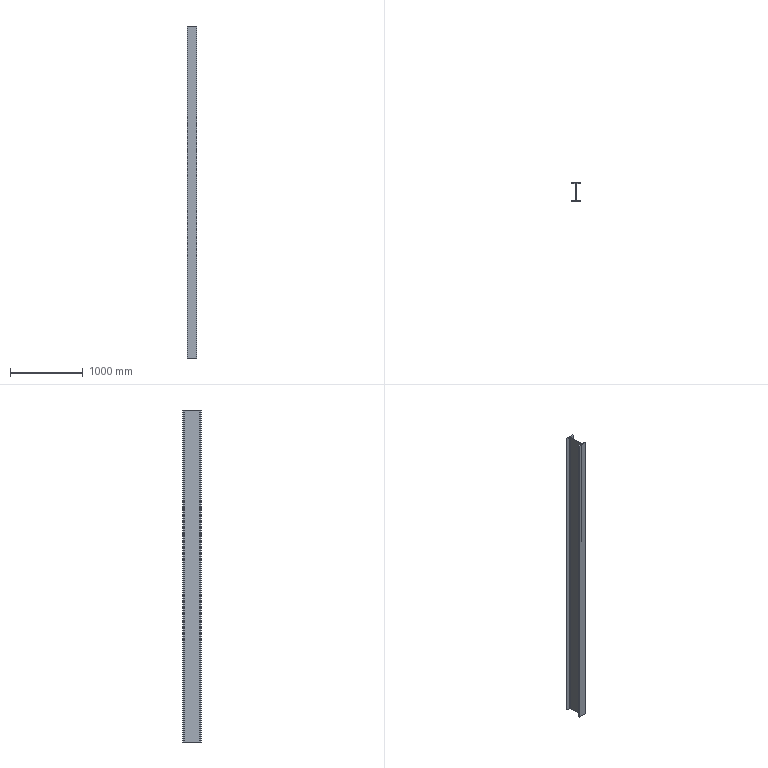Part | SolidWorks | features Extrusion 1 | 1 solid | 18 faces | box 125 x 250 x 4570 mm | volume 16895007 mm3 | plane 14 | cylinder 4 | commonest cylinder face diameters 16 x4
STEP:
#1=CARTESIAN_POINT('',(-62.5,9.,0.));
#2=VERTEX_POINT('',#1);
#3=CARTESIAN_POINT('',(-62.5,0.,0.));
#4=VERTEX_POINT('',#3);
#5=CARTESIAN_POINT('',(-62.5,0.,0.));
#6=DIRECTION('',(0.,-1.,0.));
#7=VECTOR('',#6,1000.);
#8=LINE('',#5,#7);
#9=EDGE_CURVE('',#2,#4,#8,.T.);
#10=ORIENTED_EDGE('',*,*,#9,.T.);
#11=CARTESIAN_POINT('',(-62.5,0.,4570.));
#12=VERTEX_POINT('',#11);
#13=CARTESIAN_POINT('',(-62.5,0.,4570.));
#14=DIRECTION('',(0.,0.,-1.));
#15=VECTOR('',#14,1000.);
#16=LINE('',#13,#15);
#17=EDGE_CURVE('',#12,#4,#16,.T.);
#18=ORIENTED_EDGE('',*,*,#17,.F.);
#19=CARTESIAN_POINT('',(-62.5,9.,4570.));
#20=VERTEX_POINT('',#19);
#21=CARTESIAN_POINT('',(-62.5,0.,4570.));
#22=DIRECTION('',(0.,-1.,0.));
#23=VECTOR('',#22,1000.);
#24=LINE('',#21,#23);
#25=EDGE_CURVE('',#20,#12,#24,.T.);
#26=ORIENTED_EDGE('',*,*,#25,.F.);
#27=CARTESIAN_POINT('',(-62.5,9.,4570.));
#28=DIRECTION('',(0.,0.,-1.));
#29=VECTOR('',#28,1000.);
#30=LINE('',#27,#29);
#31=EDGE_CURVE('',#20,#2,#30,.T.);
#32=ORIENTED_EDGE('',*,*,#31,.T.);
#33=EDGE_LOOP('',(#10,#18,#26,#32));
#34=FACE_OUTER_BOUND('',#33,.T.);
#35=CARTESIAN_POINT('',(-62.5,0.,4570.));
#36=DIRECTION('',(1.,0.,0.));
#37=DIRECTION('',(0.,0.,-1.));
#38=AXIS2_PLACEMENT_3D('',#35,#36,#37);
#39=PLANE('',#38);
#40=ADVANCED_FACE('',(#34),#39,.F.);
#41=CARTESIAN_POINT('',(62.5,0.,0.));
#42=VERTEX_POINT('',#41);
#43=CARTESIAN_POINT('',(62.5,0.,0.));
#44=DIRECTION('',(1.,0.,0.));
#45=VECTOR('',#44,1000.);
#46=LINE('',#43,#45);
#47=EDGE_CURVE('',#4,#42,#46,.T.);
#48=ORIENTED_EDGE('',*,*,#47,.T.);
#49=CARTESIAN_POINT('',(62.5,0.,4570.));
#50=VERTEX_POINT('',#49);
#51=CARTESIAN_POINT('',(62.5,0.,4570.));
#52=DIRECTION('',(0.,0.,-1.));
#53=VECTOR('',#52,1000.);
#54=LINE('',#51,#53);
#55=EDGE_CURVE('',#50,#42,#54,.T.);
#56=ORIENTED_EDGE('',*,*,#55,.F.);
#57=CARTESIAN_POINT('',(62.5,0.,4570.));
#58=DIRECTION('',(1.,0.,0.));
#59=VECTOR('',#58,1000.);
#60=LINE('',#57,#59);
#61=EDGE_CURVE('',#12,#50,#60,.T.);
#62=ORIENTED_EDGE('',*,*,#61,.F.);
#63=ORIENTED_EDGE('',*,*,#17,.T.);
#64=EDGE_LOOP('',(#48,#56,#62,#63));
#65=FACE_OUTER_BOUND('',#64,.T.);
#66=CARTESIAN_POINT('',(62.5,0.,4570.));
#67=DIRECTION('',(0.,1.,0.));
#68=DIRECTION('',(0.,0.,1.));
#69=AXIS2_PLACEMENT_3D('',#66,#67,#68);
#70=PLANE('',#69);
#71=ADVANCED_FACE('',(#65),#70,.F.);
#72=CARTESIAN_POINT('',(62.5,9.,0.));
#73=VERTEX_POINT('',#72);
#74=CARTESIAN_POINT('',(62.5,0.,0.));
#75=DIRECTION('',(0.,1.,0.));
#76=VECTOR('',#75,1000.);
#77=LINE('',#74,#76);
#78=EDGE_CURVE('',#42,#73,#77,.T.);
#79=ORIENTED_EDGE('',*,*,#78,.T.);
#80=CARTESIAN_POINT('',(62.5,9.,4570.));
#81=VERTEX_POINT('',#80);
#82=CARTESIAN_POINT('',(62.5,9.,4570.));
#83=DIRECTION('',(0.,0.,-1.));
#84=VECTOR('',#83,1000.);
#85=LINE('',#82,#84);
#86=EDGE_CURVE('',#81,#73,#85,.T.);
#87=ORIENTED_EDGE('',*,*,#86,.F.);
#88=CARTESIAN_POINT('',(62.5,0.,4570.));
#89=DIRECTION('',(0.,1.,0.));
#90=VECTOR('',#89,1000.);
#91=LINE('',#88,#90);
#92=EDGE_CURVE('',#50,#81,#91,.T.);
#93=ORIENTED_EDGE('',*,*,#92,.F.);
#94=ORIENTED_EDGE('',*,*,#55,.T.);
#95=EDGE_LOOP('',(#79,#87,#93,#94));
#96=FACE_OUTER_BOUND('',#95,.T.);
#97=CARTESIAN_POINT('',(62.5,0.,4570.));
#98=DIRECTION('',(-1.,0.,0.));
#99=DIRECTION('',(0.,0.,1.));
#100=AXIS2_PLACEMENT_3D('',#97,#98,#99);
#101=PLANE('',#100);
#102=ADVANCED_FACE('',(#96),#101,.F.);
#103=CARTESIAN_POINT('',(11.,9.,0.));
#104=VERTEX_POINT('',#103);
#105=CARTESIAN_POINT('',(62.5,9.,0.));
#106=DIRECTION('',(-1.,0.,0.));
#107=VECTOR('',#106,1000.);
#108=LINE('',#105,#107);
#109=EDGE_CURVE('',#73,#104,#108,.T.);
#110=ORIENTED_EDGE('',*,*,#109,.T.);
#111=CARTESIAN_POINT('',(11.,9.,4570.));
#112=VERTEX_POINT('',#111);
#113=CARTESIAN_POINT('',(11.,9.,4570.));
#114=DIRECTION('',(0.,0.,-1.));
#115=VECTOR('',#114,1000.);
#116=LINE('',#113,#115);
#117=EDGE_CURVE('',#112,#104,#116,.T.);
#118=ORIENTED_EDGE('',*,*,#117,.F.);
#119=CARTESIAN_POINT('',(62.5,9.,4570.));
#120=DIRECTION('',(-1.,0.,0.));
#121=VECTOR('',#120,1000.);
#122=LINE('',#119,#121);
#123=EDGE_CURVE('',#81,#112,#122,.T.);
#124=ORIENTED_EDGE('',*,*,#123,.F.);
#125=ORIENTED_EDGE('',*,*,#86,.T.);
#126=EDGE_LOOP('',(#110,#118,#124,#125));
#127=FACE_OUTER_BOUND('',#126,.T.);
#128=CARTESIAN_POINT('',(62.5,9.,4570.));
#129=DIRECTION('',(0.,-1.,0.));
#130=DIRECTION('',(0.,0.,-1.));
#131=AXIS2_PLACEMENT_3D('',#128,#129,#130);
#132=PLANE('',#131);
#133=ADVANCED_FACE('',(#127),#132,.F.);
#134=CARTESIAN_POINT('',(3.,17.,0.));
#135=VERTEX_POINT('',#134);
#136=CARTESIAN_POINT('',(11.,17.,0.));
#137=DIRECTION('',(0.,0.,-1.));
#138=DIRECTION('',(-1.,0.,0.));
#139=AXIS2_PLACEMENT_3D('',#136,#137,#138);
#140=CIRCLE('',#139,8.);
#141=EDGE_CURVE('',#104,#135,#140,.T.);
#142=ORIENTED_EDGE('',*,*,#141,.T.);
#143=CARTESIAN_POINT('',(3.,17.,4570.));
#144=VERTEX_POINT('',#143);
#145=CARTESIAN_POINT('',(3.,17.,4570.));
#146=DIRECTION('',(0.,0.,-1.));
#147=VECTOR('',#146,1000.);
#148=LINE('',#145,#147);
#149=EDGE_CURVE('',#144,#135,#148,.T.);
#150=ORIENTED_EDGE('',*,*,#149,.F.);
#151=CARTESIAN_POINT('',(11.,17.,4570.));
#152=DIRECTION('',(0.,0.,-1.));
#153=DIRECTION('',(-1.,0.,0.));
#154=AXIS2_PLACEMENT_3D('',#151,#152,#153);
#155=CIRCLE('',#154,8.);
#156=EDGE_CURVE('',#112,#144,#155,.T.);
#157=ORIENTED_EDGE('',*,*,#156,.F.);
#158=ORIENTED_EDGE('',*,*,#117,.T.);
#159=EDGE_LOOP('',(#142,#150,#157,#158));
#160=FACE_OUTER_BOUND('',#159,.T.);
#161=CARTESIAN_POINT('',(11.,17.,4570.));
#162=DIRECTION('',(0.,0.,-1.));
#163=DIRECTION('',(-1.,0.,0.));
#164=AXIS2_PLACEMENT_3D('',#161,#162,#163);
#165=CYLINDRICAL_SURFACE('',#164,8.);
#166=ADVANCED_FACE('',(#160),#165,.F.);
#167=CARTESIAN_POINT('',(3.,233.,0.));
#168=VERTEX_POINT('',#167);
#169=CARTESIAN_POINT('',(3.,17.,0.));
#170=DIRECTION('',(0.,1.,0.));
#171=VECTOR('',#170,1000.);
#172=LINE('',#169,#171);
#173=EDGE_CURVE('',#135,#168,#172,.T.);
#174=ORIENTED_EDGE('',*,*,#173,.T.);
#175=CARTESIAN_POINT('',(3.,233.,4570.));
#176=VERTEX_POINT('',#175);
#177=CARTESIAN_POINT('',(3.,233.,4570.));
#178=DIRECTION('',(0.,0.,-1.));
#179=VECTOR('',#178,1000.);
#180=LINE('',#177,#179);
#181=EDGE_CURVE('',#176,#168,#180,.T.);
#182=ORIENTED_EDGE('',*,*,#181,.F.);
#183=CARTESIAN_POINT('',(3.,17.,4570.));
#184=DIRECTION('',(0.,1.,0.));
#185=VECTOR('',#184,1000.);
#186=LINE('',#183,#185);
#187=EDGE_CURVE('',#144,#176,#186,.T.);
#188=ORIENTED_EDGE('',*,*,#187,.F.);
#189=ORIENTED_EDGE('',*,*,#149,.T.);
#190=EDGE_LOOP('',(#174,#182,#188,#189));
#191=FACE_OUTER_BOUND('',#190,.T.);
#192=CARTESIAN_POINT('',(3.,17.,4570.));
#193=DIRECTION('',(-1.,0.,0.));
#194=DIRECTION('',(0.,-1.,0.));
#195=AXIS2_PLACEMENT_3D('',#192,#193,#194);
#196=PLANE('',#195);
#197=ADVANCED_FACE('',(#191),#196,.F.);
#198=CARTESIAN_POINT('',(11.,241.,0.));
#199=VERTEX_POINT('',#198);
#200=CARTESIAN_POINT('',(11.,233.,0.));
#201=DIRECTION('',(0.,0.,-1.));
#202=DIRECTION('',(-1.,0.,0.));
#203=AXIS2_PLACEMENT_3D('',#200,#201,#202);
#204=CIRCLE('',#203,8.);
#205=EDGE_CURVE('',#168,#199,#204,.T.);
#206=ORIENTED_EDGE('',*,*,#205,.T.);
#207=CARTESIAN_POINT('',(11.,241.,4570.));
#208=VERTEX_POINT('',#207);
#209=CARTESIAN_POINT('',(11.,241.,4570.));
#210=DIRECTION('',(0.,0.,-1.));
#211=VECTOR('',#210,1000.);
#212=LINE('',#209,#211);
#213=EDGE_CURVE('',#208,#199,#212,.T.);
#214=ORIENTED_EDGE('',*,*,#213,.F.);
#215=CARTESIAN_POINT('',(11.,233.,4570.));
#216=DIRECTION('',(0.,0.,-1.));
#217=DIRECTION('',(-1.,0.,0.));
#218=AXIS2_PLACEMENT_3D('',#215,#216,#217);
#219=CIRCLE('',#218,8.);
#220=EDGE_CURVE('',#176,#208,#219,.T.);
#221=ORIENTED_EDGE('',*,*,#220,.F.);
#222=ORIENTED_EDGE('',*,*,#181,.T.);
#223=EDGE_LOOP('',(#206,#214,#221,#222));
#224=FACE_OUTER_BOUND('',#223,.T.);
#225=CARTESIAN_POINT('',(11.,233.,4570.));
#226=DIRECTION('',(0.,0.,-1.));
#227=DIRECTION('',(-1.,0.,0.));
#228=AXIS2_PLACEMENT_3D('',#225,#226,#227);
#229=CYLINDRICAL_SURFACE('',#228,8.);
#230=ADVANCED_FACE('',(#224),#229,.F.);
#231=CARTESIAN_POINT('',(62.5,241.,0.));
#232=VERTEX_POINT('',#231);
#233=CARTESIAN_POINT('',(11.,241.,0.));
#234=DIRECTION('',(1.,0.,0.));
#235=VECTOR('',#234,1000.);
#236=LINE('',#233,#235);
#237=EDGE_CURVE('',#199,#232,#236,.T.);
#238=ORIENTED_EDGE('',*,*,#237,.T.);
#239=CARTESIAN_POINT('',(62.5,241.,4570.));
#240=VERTEX_POINT('',#239);
#241=CARTESIAN_POINT('',(62.5,241.,4570.));
#242=DIRECTION('',(0.,0.,-1.));
#243=VECTOR('',#242,1000.);
#244=LINE('',#241,#243);
#245=EDGE_CURVE('',#240,#232,#244,.T.);
#246=ORIENTED_EDGE('',*,*,#245,.F.);
#247=CARTESIAN_POINT('',(11.,241.,4570.));
#248=DIRECTION('',(1.,0.,0.));
#249=VECTOR('',#248,1000.);
#250=LINE('',#247,#249);
#251=EDGE_CURVE('',#208,#240,#250,.T.);
#252=ORIENTED_EDGE('',*,*,#251,.F.);
#253=ORIENTED_EDGE('',*,*,#213,.T.);
#254=EDGE_LOOP('',(#238,#246,#252,#253));
#255=FACE_OUTER_BOUND('',#254,.T.);
#256=CARTESIAN_POINT('',(11.,241.,4570.));
#257=DIRECTION('',(0.,1.,0.));
#258=DIRECTION('',(0.,0.,1.));
#259=AXIS2_PLACEMENT_3D('',#256,#257,#258);
#260=PLANE('',#259);
#261=ADVANCED_FACE('',(#255),#260,.F.);
#262=CARTESIAN_POINT('',(62.5,250.,0.));
#263=VERTEX_POINT('',#262);
#264=CARTESIAN_POINT('',(62.5,241.,0.));
#265=DIRECTION('',(0.,1.,0.));
#266=VECTOR('',#265,1000.);
#267=LINE('',#264,#266);
#268=EDGE_CURVE('',#232,#263,#267,.T.);
#269=ORIENTED_EDGE('',*,*,#268,.T.);
#270=CARTESIAN_POINT('',(62.5,250.,4570.));
#271=VERTEX_POINT('',#270);
#272=CARTESIAN_POINT('',(62.5,250.,4570.));
#273=DIRECTION('',(0.,0.,-1.));
#274=VECTOR('',#273,1000.);
#275=LINE('',#272,#274);
#276=EDGE_CURVE('',#271,#263,#275,.T.);
#277=ORIENTED_EDGE('',*,*,#276,.F.);
#278=CARTESIAN_POINT('',(62.5,241.,4570.));
#279=DIRECTION('',(0.,1.,0.));
#280=VECTOR('',#279,1000.);
#281=LINE('',#278,#280);
#282=EDGE_CURVE('',#240,#271,#281,.T.);
#283=ORIENTED_EDGE('',*,*,#282,.F.);
#284=ORIENTED_EDGE('',*,*,#245,.T.);
#285=EDGE_LOOP('',(#269,#277,#283,#284));
#286=FACE_OUTER_BOUND('',#285,.T.);
#287=CARTESIAN_POINT('',(62.5,241.,4570.));
#288=DIRECTION('',(-1.,0.,0.));
#289=DIRECTION('',(0.,0.,1.));
#290=AXIS2_PLACEMENT_3D('',#287,#288,#289);
#291=PLANE('',#290);
#292=ADVANCED_FACE('',(#286),#291,.F.);
#293=CARTESIAN_POINT('',(-62.5,250.,0.));
#294=VERTEX_POINT('',#293);
#295=CARTESIAN_POINT('',(-62.5,250.,0.));
#296=DIRECTION('',(-1.,0.,0.));
#297=VECTOR('',#296,1000.);
#298=LINE('',#295,#297);
#299=EDGE_CURVE('',#263,#294,#298,.T.);
#300=ORIENTED_EDGE('',*,*,#299,.T.);
#301=CARTESIAN_POINT('',(-62.5,250.,4570.));
#302=VERTEX_POINT('',#301);
#303=CARTESIAN_POINT('',(-62.5,250.,4570.));
#304=DIRECTION('',(0.,0.,-1.));
#305=VECTOR('',#304,1000.);
#306=LINE('',#303,#305);
#307=EDGE_CURVE('',#302,#294,#306,.T.);
#308=ORIENTED_EDGE('',*,*,#307,.F.);
#309=CARTESIAN_POINT('',(-62.5,250.,4570.));
#310=DIRECTION('',(-1.,0.,0.));
#311=VECTOR('',#310,1000.);
#312=LINE('',#309,#311);
#313=EDGE_CURVE('',#271,#302,#312,.T.);
#314=ORIENTED_EDGE('',*,*,#313,.F.);
#315=ORIENTED_EDGE('',*,*,#276,.T.);
#316=EDGE_LOOP('',(#300,#308,#314,#315));
#317=FACE_OUTER_BOUND('',#316,.T.);
#318=CARTESIAN_POINT('',(-62.5,250.,4570.));
#319=DIRECTION('',(0.,-1.,0.));
#320=DIRECTION('',(1.,0.,0.));
#321=AXIS2_PLACEMENT_3D('',#318,#319,#320);
#322=PLANE('',#321);
#323=ADVANCED_FACE('',(#317),#322,.F.);
#324=CARTESIAN_POINT('',(-62.5,241.,0.));
#325=VERTEX_POINT('',#324);
#326=CARTESIAN_POINT('',(-62.5,241.,0.));
#327=DIRECTION('',(0.,-1.,0.));
#328=VECTOR('',#327,1000.);
#329=LINE('',#326,#328);
#330=EDGE_CURVE('',#294,#325,#329,.T.);
#331=ORIENTED_EDGE('',*,*,#330,.T.);
#332=CARTESIAN_POINT('',(-62.5,241.,4570.));
#333=VERTEX_POINT('',#332);
#334=CARTESIAN_POINT('',(-62.5,241.,4570.));
#335=DIRECTION('',(0.,0.,-1.));
#336=VECTOR('',#335,1000.);
#337=LINE('',#334,#336);
#338=EDGE_CURVE('',#333,#325,#337,.T.);
#339=ORIENTED_EDGE('',*,*,#338,.F.);
#340=CARTESIAN_POINT('',(-62.5,241.,4570.));
#341=DIRECTION('',(0.,-1.,0.));
#342=VECTOR('',#341,1000.);
#343=LINE('',#340,#342);
#344=EDGE_CURVE('',#302,#333,#343,.T.);
#345=ORIENTED_EDGE('',*,*,#344,.F.);
#346=ORIENTED_EDGE('',*,*,#307,.T.);
#347=EDGE_LOOP('',(#331,#339,#345,#346));
#348=FACE_OUTER_BOUND('',#347,.T.);
#349=CARTESIAN_POINT('',(-62.5,241.,4570.));
#350=DIRECTION('',(1.,0.,0.));
#351=DIRECTION('',(0.,0.,-1.));
#352=AXIS2_PLACEMENT_3D('',#349,#350,#351);
#353=PLANE('',#352);
#354=ADVANCED_FACE('',(#348),#353,.F.);
#355=CARTESIAN_POINT('',(-11.,241.,0.));
#356=VERTEX_POINT('',#355);
#357=CARTESIAN_POINT('',(-11.,241.,0.));
#358=DIRECTION('',(1.,0.,0.));
#359=VECTOR('',#358,1000.);
#360=LINE('',#357,#359);
#361=EDGE_CURVE('',#325,#356,#360,.T.);
#362=ORIENTED_EDGE('',*,*,#361,.T.);
#363=CARTESIAN_POINT('',(-11.,241.,4570.));
#364=VERTEX_POINT('',#363);
#365=CARTESIAN_POINT('',(-11.,241.,4570.));
#366=DIRECTION('',(0.,0.,-1.));
#367=VECTOR('',#366,1000.);
#368=LINE('',#365,#367);
#369=EDGE_CURVE('',#364,#356,#368,.T.);
#370=ORIENTED_EDGE('',*,*,#369,.F.);
#371=CARTESIAN_POINT('',(-11.,241.,4570.));
#372=DIRECTION('',(1.,0.,0.));
#373=VECTOR('',#372,1000.);
#374=LINE('',#371,#373);
#375=EDGE_CURVE('',#333,#364,#374,.T.);
#376=ORIENTED_EDGE('',*,*,#375,.F.);
#377=ORIENTED_EDGE('',*,*,#338,.T.);
#378=EDGE_LOOP('',(#362,#370,#376,#377));
#379=FACE_OUTER_BOUND('',#378,.T.);
#380=CARTESIAN_POINT('',(-11.,241.,4570.));
#381=DIRECTION('',(0.,1.,0.));
#382=DIRECTION('',(0.,0.,1.));
#383=AXIS2_PLACEMENT_3D('',#380,#381,#382);
#384=PLANE('',#383);
#385=ADVANCED_FACE('',(#379),#384,.F.);
#386=CARTESIAN_POINT('',(-3.,233.,0.));
#387=VERTEX_POINT('',#386);
#388=CARTESIAN_POINT('',(-11.,233.,0.));
#389=DIRECTION('',(0.,0.,-1.));
#390=DIRECTION('',(1.,0.,0.));
#391=AXIS2_PLACEMENT_3D('',#388,#389,#390);
#392=CIRCLE('',#391,8.);
#393=EDGE_CURVE('',#356,#387,#392,.T.);
#394=ORIENTED_EDGE('',*,*,#393,.T.);
#395=CARTESIAN_POINT('',(-3.,233.,4570.));
#396=VERTEX_POINT('',#395);
#397=CARTESIAN_POINT('',(-3.,233.,4570.));
#398=DIRECTION('',(0.,0.,-1.));
#399=VECTOR('',#398,1000.);
#400=LINE('',#397,#399);
#401=EDGE_CURVE('',#396,#387,#400,.T.);
#402=ORIENTED_EDGE('',*,*,#401,.F.);
#403=CARTESIAN_POINT('',(-11.,233.,4570.));
#404=DIRECTION('',(0.,0.,-1.));
#405=DIRECTION('',(1.,0.,0.));
#406=AXIS2_PLACEMENT_3D('',#403,#404,#405);
#407=CIRCLE('',#406,8.);
#408=EDGE_CURVE('',#364,#396,#407,.T.);
#409=ORIENTED_EDGE('',*,*,#408,.F.);
#410=ORIENTED_EDGE('',*,*,#369,.T.);
#411=EDGE_LOOP('',(#394,#402,#409,#410));
#412=FACE_OUTER_BOUND('',#411,.T.);
#413=CARTESIAN_POINT('',(-11.,233.,4570.));
#414=DIRECTION('',(0.,0.,-1.));
#415=DIRECTION('',(-1.,0.,0.));
#416=AXIS2_PLACEMENT_3D('',#413,#414,#415);
#417=CYLINDRICAL_SURFACE('',#416,8.);
#418=ADVANCED_FACE('',(#412),#417,.F.);
#419=CARTESIAN_POINT('',(-3.,17.,0.));
#420=VERTEX_POINT('',#419);
#421=CARTESIAN_POINT('',(-3.,17.,0.));
#422=DIRECTION('',(0.,-1.,0.));
#423=VECTOR('',#422,1000.);
#424=LINE('',#421,#423);
#425=EDGE_CURVE('',#387,#420,#424,.T.);
#426=ORIENTED_EDGE('',*,*,#425,.T.);
#427=CARTESIAN_POINT('',(-3.,17.,4570.));
#428=VERTEX_POINT('',#427);
#429=CARTESIAN_POINT('',(-3.,17.,4570.));
#430=DIRECTION('',(0.,0.,-1.));
#431=VECTOR('',#430,1000.);
#432=LINE('',#429,#431);
#433=EDGE_CURVE('',#428,#420,#432,.T.);
#434=ORIENTED_EDGE('',*,*,#433,.F.);
#435=CARTESIAN_POINT('',(-3.,17.,4570.));
#436=DIRECTION('',(0.,-1.,0.));
#437=VECTOR('',#436,1000.);
#438=LINE('',#435,#437);
#439=EDGE_CURVE('',#396,#428,#438,.T.);
#440=ORIENTED_EDGE('',*,*,#439,.F.);
#441=ORIENTED_EDGE('',*,*,#401,.T.);
#442=EDGE_LOOP('',(#426,#434,#440,#441));
#443=FACE_OUTER_BOUND('',#442,.T.);
#444=CARTESIAN_POINT('',(-3.,17.,4570.));
#445=DIRECTION('',(1.,0.,0.));
#446=DIRECTION('',(0.,1.,0.));
#447=AXIS2_PLACEMENT_3D('',#444,#445,#446);
#448=PLANE('',#447);
#449=ADVANCED_FACE('',(#443),#448,.F.);
#450=CARTESIAN_POINT('',(-11.,9.,0.));
#451=VERTEX_POINT('',#450);
#452=CARTESIAN_POINT('',(-11.,17.,0.));
#453=DIRECTION('',(0.,0.,-1.));
#454=DIRECTION('',(-1.,0.,0.));
#455=AXIS2_PLACEMENT_3D('',#452,#453,#454);
#456=CIRCLE('',#455,8.);
#457=EDGE_CURVE('',#420,#451,#456,.T.);
#458=ORIENTED_EDGE('',*,*,#457,.T.);
#459=CARTESIAN_POINT('',(-11.,9.,4570.));
#460=VERTEX_POINT('',#459);
#461=CARTESIAN_POINT('',(-11.,9.,4570.));
#462=DIRECTION('',(0.,0.,-1.));
#463=VECTOR('',#462,1000.);
#464=LINE('',#461,#463);
#465=EDGE_CURVE('',#460,#451,#464,.T.);
#466=ORIENTED_EDGE('',*,*,#465,.F.);
#467=CARTESIAN_POINT('',(-11.,17.,4570.));
#468=DIRECTION('',(0.,0.,-1.));
#469=DIRECTION('',(-1.,0.,0.));
#470=AXIS2_PLACEMENT_3D('',#467,#468,#469);
#471=CIRCLE('',#470,8.);
#472=EDGE_CURVE('',#428,#460,#471,.T.);
#473=ORIENTED_EDGE('',*,*,#472,.F.);
#474=ORIENTED_EDGE('',*,*,#433,.T.);
#475=EDGE_LOOP('',(#458,#466,#473,#474));
#476=FACE_OUTER_BOUND('',#475,.T.);
#477=CARTESIAN_POINT('',(-11.,17.,4570.));
#478=DIRECTION('',(0.,0.,-1.));
#479=DIRECTION('',(-1.,0.,0.));
#480=AXIS2_PLACEMENT_3D('',#477,#478,#479);
#481=CYLINDRICAL_SURFACE('',#480,8.);
#482=ADVANCED_FACE('',(#476),#481,.F.);
#483=CARTESIAN_POINT('',(-62.5,9.,0.));
#484=DIRECTION('',(-1.,0.,0.));
#485=VECTOR('',#484,1000.);
#486=LINE('',#483,#485);
#487=EDGE_CURVE('',#451,#2,#486,.T.);
#488=ORIENTED_EDGE('',*,*,#487,.T.);
#489=ORIENTED_EDGE('',*,*,#31,.F.);
#490=CARTESIAN_POINT('',(-62.5,9.,4570.));
#491=DIRECTION('',(-1.,0.,0.));
#492=VECTOR('',#491,1000.);
#493=LINE('',#490,#492);
#494=EDGE_CURVE('',#460,#20,#493,.T.);
#495=ORIENTED_EDGE('',*,*,#494,.F.);
#496=ORIENTED_EDGE('',*,*,#465,.T.);
#497=EDGE_LOOP('',(#488,#489,#495,#496));
#498=FACE_OUTER_BOUND('',#497,.T.);
#499=CARTESIAN_POINT('',(-62.5,9.,4570.));
#500=DIRECTION('',(0.,-1.,0.));
#501=DIRECTION('',(0.,0.,-1.));
#502=AXIS2_PLACEMENT_3D('',#499,#500,#501);
#503=PLANE('',#502);
#504=ADVANCED_FACE('',(#498),#503,.F.);
#505=ORIENTED_EDGE('',*,*,#25,.T.);
#506=ORIENTED_EDGE('',*,*,#61,.T.);
#507=ORIENTED_EDGE('',*,*,#92,.T.);
#508=ORIENTED_EDGE('',*,*,#123,.T.);
#509=ORIENTED_EDGE('',*,*,#156,.T.);
#510=ORIENTED_EDGE('',*,*,#187,.T.);
#511=ORIENTED_EDGE('',*,*,#220,.T.);
#512=ORIENTED_EDGE('',*,*,#251,.T.);
#513=ORIENTED_EDGE('',*,*,#282,.T.);
#514=ORIENTED_EDGE('',*,*,#313,.T.);
#515=ORIENTED_EDGE('',*,*,#344,.T.);
#516=ORIENTED_EDGE('',*,*,#375,.T.);
#517=ORIENTED_EDGE('',*,*,#408,.T.);
#518=ORIENTED_EDGE('',*,*,#439,.T.);
#519=ORIENTED_EDGE('',*,*,#472,.T.);
#520=ORIENTED_EDGE('',*,*,#494,.T.);
#521=EDGE_LOOP('',(#505,#506,#507,#508,#509,#510,#511,#512,#513,#514,#515,#516,#517,#518,#519,#520));
#522=FACE_OUTER_BOUND('',#521,.T.);
#523=CARTESIAN_POINT('',(-11.,17.,4570.));
#524=DIRECTION('',(0.,0.,-1.));
#525=DIRECTION('',(-1.,0.,0.));
#526=AXIS2_PLACEMENT_3D('',#523,#524,#525);
#527=PLANE('',#526);
#528=ADVANCED_FACE('',(#522),#527,.F.);
#529=ORIENTED_EDGE('',*,*,#9,.F.);
#530=ORIENTED_EDGE('',*,*,#487,.F.);
#531=ORIENTED_EDGE('',*,*,#457,.F.);
#532=ORIENTED_EDGE('',*,*,#425,.F.);
#533=ORIENTED_EDGE('',*,*,#393,.F.);
#534=ORIENTED_EDGE('',*,*,#361,.F.);
#535=ORIENTED_EDGE('',*,*,#330,.F.);
#536=ORIENTED_EDGE('',*,*,#299,.F.);
#537=ORIENTED_EDGE('',*,*,#268,.F.);
#538=ORIENTED_EDGE('',*,*,#237,.F.);
#539=ORIENTED_EDGE('',*,*,#205,.F.);
#540=ORIENTED_EDGE('',*,*,#173,.F.);
#541=ORIENTED_EDGE('',*,*,#141,.F.);
#542=ORIENTED_EDGE('',*,*,#109,.F.);
#543=ORIENTED_EDGE('',*,*,#78,.F.);
#544=ORIENTED_EDGE('',*,*,#47,.F.);
#545=EDGE_LOOP('',(#529,#530,#531,#532,#533,#534,#535,#536,#537,#538,#539,#540,#541,#542,#543,#544));
#546=FACE_OUTER_BOUND('',#545,.T.);
#547=CARTESIAN_POINT('',(-11.,17.,0.));
#548=DIRECTION('',(0.,0.,-1.));
#549=DIRECTION('',(-1.,0.,0.));
#550=AXIS2_PLACEMENT_3D('',#547,#548,#549);
#551=PLANE('',#550);
#552=ADVANCED_FACE('',(#546),#551,.T.);
#553=CLOSED_SHELL('',(#40,#71,#102,#133,#166,#197,#230,#261,#292,#323,#354,#385,#418,#449,#482,#504,#528,#552));
#554=MANIFOLD_SOLID_BREP('',#553);
#555=CARTESIAN_POINT('',(0.,0.,0.));
#556=DIRECTION('',(0.,0.,1.));
#557=DIRECTION('',(1.,0.,0.));
#558=AXIS2_PLACEMENT_3D('',#555,#556,#557);
#559=(LENGTH_UNIT()NAMED_UNIT(*)SI_UNIT(.MILLI.,.METRE.));
#560=UNCERTAINTY_MEASURE_WITH_UNIT(LENGTH_MEASURE(0.00001),#559,'','');
#561=(NAMED_UNIT(*)PLANE_ANGLE_UNIT()SI_UNIT($,.RADIAN.));
#562=(NAMED_UNIT(*)SI_UNIT($,.STERADIAN.)SOLID_ANGLE_UNIT());
#563=(GEOMETRIC_REPRESENTATION_CONTEXT(3)GLOBAL_UNCERTAINTY_ASSIGNED_CONTEXT((#560))GLOBAL_UNIT_ASSIGNED_CONTEXT((#559,#561,#562))REPRESENTATION_CONTEXT('',''));
#564=ADVANCED_BREP_SHAPE_REPRESENTATION('',(#554,#558),#563);